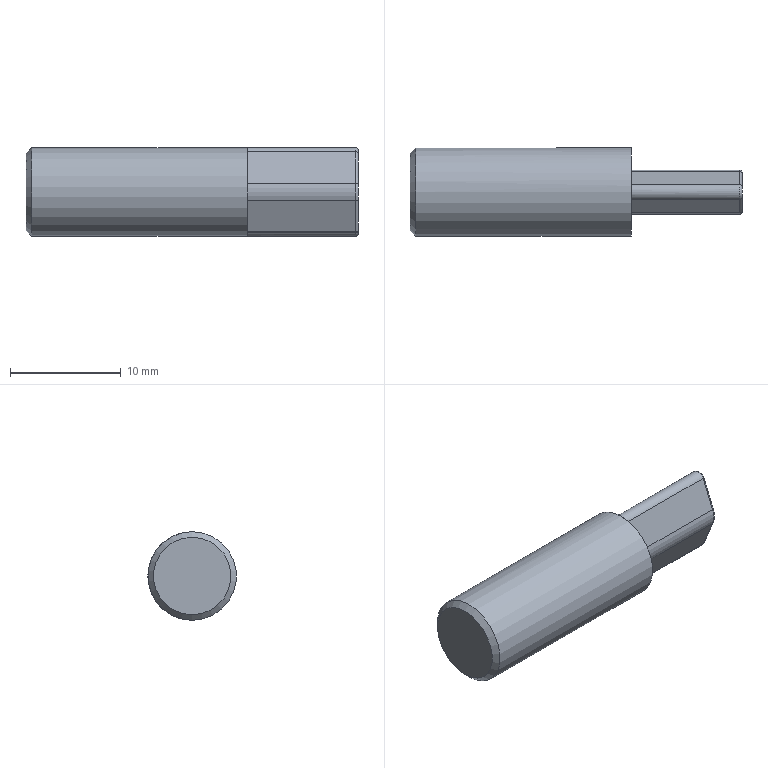Part | NX | features DATUM_CSYS 3, BLEND 2, EXTRUDE 2, SKETCH 2, CHAMFER 1 | 1 solid | 26 faces | box 30 x 8 x 8 mm | volume 1212 mm3 | cylinder 11 | plane 8 | torus 4 | sphere 2 | cone 1 | commonest cylinder face diameters 0.4 x6 1.5 x2 4 x2 8 x1
STEP:
#1=CARTESIAN_POINT('',(20.,0.,4.));
#2=VERTEX_POINT('',#1);
#3=CARTESIAN_POINT('',(20.,-0.6495,3.625));
#4=VERTEX_POINT('',#3);
#5=CARTESIAN_POINT('',(20.,0.,3.25));
#6=DIRECTION('',(1.,0.,0.));
#7=DIRECTION('',(0.,1.,0.));
#8=AXIS2_PLACEMENT_3D('',#5,#6,#7);
#9=CIRCLE('',#8,0.75);
#10=EDGE_CURVE('',#2,#4,#9,.T.);
#11=ORIENTED_EDGE('',*,*,#10,.F.);
#12=CARTESIAN_POINT('',(20.,0.,-4.));
#13=VERTEX_POINT('',#12);
#14=CARTESIAN_POINT('',(20.,0.,0.));
#15=DIRECTION('',(1.,0.,0.));
#16=DIRECTION('',(0.,1.,0.));
#17=AXIS2_PLACEMENT_3D('',#14,#15,#16);
#18=CIRCLE('',#17,4.);
#19=EDGE_CURVE('',#2,#13,#18,.T.);
#20=ORIENTED_EDGE('',*,*,#19,.T.);
#21=CARTESIAN_POINT('',(20.,-0.6414,-3.639));
#22=VERTEX_POINT('',#21);
#23=CARTESIAN_POINT('',(20.,0.,-3.25));
#24=DIRECTION('',(1.,0.,0.));
#25=DIRECTION('',(0.,1.,0.));
#26=AXIS2_PLACEMENT_3D('',#23,#24,#25);
#27=CIRCLE('',#26,0.75);
#28=EDGE_CURVE('',#22,#13,#27,.T.);
#29=ORIENTED_EDGE('',*,*,#28,.F.);
#30=CARTESIAN_POINT('',(20.,-0.6548,-3.612));
#31=VERTEX_POINT('',#30);
#32=CARTESIAN_POINT('',(20.,-0.4703,-3.535));
#33=DIRECTION('',(1.,0.,0.));
#34=DIRECTION('',(0.,0.,-1.));
#35=AXIS2_PLACEMENT_3D('',#32,#33,#34);
#36=CIRCLE('',#35,0.2);
#37=EDGE_CURVE('',#22,#31,#36,.F.);
#38=ORIENTED_EDGE('',*,*,#37,.T.);
#39=CARTESIAN_POINT('',(20.,-1.845,-0.7729));
#40=VERTEX_POINT('',#39);
#41=CARTESIAN_POINT('',(20.,-1.845,-0.7729));
#42=DIRECTION('',(0.,0.3865,-0.9223));
#43=VECTOR('',#42,1000.);
#44=LINE('',#41,#43);
#45=EDGE_CURVE('',#40,#31,#44,.T.);
#46=ORIENTED_EDGE('',*,*,#45,.F.);
#47=CARTESIAN_POINT('',(20.,-1.845,0.7729));
#48=VERTEX_POINT('',#47);
#49=CARTESIAN_POINT('',(20.,0.,0.));
#50=DIRECTION('',(1.,0.,0.));
#51=DIRECTION('',(0.,1.,0.));
#52=AXIS2_PLACEMENT_3D('',#49,#50,#51);
#53=CIRCLE('',#52,2.);
#54=EDGE_CURVE('',#48,#40,#53,.T.);
#55=ORIENTED_EDGE('',*,*,#54,.F.);
#56=CARTESIAN_POINT('',(20.,-0.6495,3.625));
#57=DIRECTION('',(0.,-0.3865,-0.9223));
#58=VECTOR('',#57,1000.);
#59=LINE('',#56,#58);
#60=EDGE_CURVE('',#4,#48,#59,.T.);
#61=ORIENTED_EDGE('',*,*,#60,.F.);
#62=EDGE_LOOP('',(#11,#20,#29,#38,#46,#55,#61));
#63=FACE_BOUND('',#62,.T.);
#64=CARTESIAN_POINT('',(20.,0.,0.));
#65=DIRECTION('',(1.,0.,0.));
#66=DIRECTION('',(0.,0.,-1.));
#67=AXIS2_PLACEMENT_3D('',#64,#65,#66);
#68=PLANE('',#67);
#69=ADVANCED_FACE('',(#63),#68,.T.);
#70=CARTESIAN_POINT('',(0.5,0.,-4.));
#71=VERTEX_POINT('',#70);
#72=CARTESIAN_POINT('',(0.5,0.,0.));
#73=DIRECTION('',(1.,0.,0.));
#74=DIRECTION('',(0.,0.,-1.));
#75=AXIS2_PLACEMENT_3D('',#72,#73,#74);
#76=CIRCLE('',#75,4.);
#77=EDGE_CURVE('',#71,#71,#76,.T.);
#78=ORIENTED_EDGE('',*,*,#77,.T.);
#79=EDGE_LOOP('',(#78));
#80=FACE_BOUND('',#79,.T.);
#81=ORIENTED_EDGE('',*,*,#19,.F.);
#82=CARTESIAN_POINT('',(20.,0.,0.));
#83=DIRECTION('',(1.,0.,0.));
#84=DIRECTION('',(0.,1.,0.));
#85=AXIS2_PLACEMENT_3D('',#82,#83,#84);
#86=CIRCLE('',#85,4.);
#87=EDGE_CURVE('',#13,#2,#86,.T.);
#88=ORIENTED_EDGE('',*,*,#87,.F.);
#89=EDGE_LOOP('',(#81,#88));
#90=FACE_BOUND('',#89,.T.);
#91=CARTESIAN_POINT('',(20.,0.,0.));
#92=DIRECTION('',(-1.,0.,0.));
#93=DIRECTION('',(0.,0.,1.));
#94=AXIS2_PLACEMENT_3D('',#91,#92,#93);
#95=CYLINDRICAL_SURFACE('',#94,4.);
#96=ADVANCED_FACE('',(#80,#90),#95,.T.);
#97=CARTESIAN_POINT('',(20.,0.6495,3.625));
#98=VERTEX_POINT('',#97);
#99=CARTESIAN_POINT('',(20.,0.,3.25));
#100=DIRECTION('',(1.,0.,0.));
#101=DIRECTION('',(0.,1.,0.));
#102=AXIS2_PLACEMENT_3D('',#99,#100,#101);
#103=CIRCLE('',#102,0.75);
#104=EDGE_CURVE('',#98,#2,#103,.T.);
#105=ORIENTED_EDGE('',*,*,#104,.F.);
#106=CARTESIAN_POINT('',(20.,1.845,0.7729));
#107=VERTEX_POINT('',#106);
#108=CARTESIAN_POINT('',(20.,1.845,0.7729));
#109=DIRECTION('',(0.,-0.3865,0.9223));
#110=VECTOR('',#109,1000.);
#111=LINE('',#108,#110);
#112=EDGE_CURVE('',#107,#98,#111,.T.);
#113=ORIENTED_EDGE('',*,*,#112,.F.);
#114=CARTESIAN_POINT('',(20.,1.845,-0.7729));
#115=VERTEX_POINT('',#114);
#116=CARTESIAN_POINT('',(20.,0.,0.));
#117=DIRECTION('',(1.,0.,0.));
#118=DIRECTION('',(0.,1.,0.));
#119=AXIS2_PLACEMENT_3D('',#116,#117,#118);
#120=CIRCLE('',#119,2.);
#121=EDGE_CURVE('',#115,#107,#120,.T.);
#122=ORIENTED_EDGE('',*,*,#121,.F.);
#123=CARTESIAN_POINT('',(20.,0.6548,-3.612));
#124=VERTEX_POINT('',#123);
#125=CARTESIAN_POINT('',(20.,0.6495,-3.625));
#126=DIRECTION('',(0.,0.3865,0.9223));
#127=VECTOR('',#126,1000.);
#128=LINE('',#125,#127);
#129=EDGE_CURVE('',#124,#115,#128,.T.);
#130=ORIENTED_EDGE('',*,*,#129,.F.);
#131=CARTESIAN_POINT('',(20.,0.6414,-3.639));
#132=VERTEX_POINT('',#131);
#133=CARTESIAN_POINT('',(20.,0.4703,-3.535));
#134=DIRECTION('',(1.,0.,0.));
#135=DIRECTION('',(0.,0.,-1.));
#136=AXIS2_PLACEMENT_3D('',#133,#134,#135);
#137=CIRCLE('',#136,0.2);
#138=EDGE_CURVE('',#124,#132,#137,.F.);
#139=ORIENTED_EDGE('',*,*,#138,.T.);
#140=CARTESIAN_POINT('',(20.,0.,-3.25));
#141=DIRECTION('',(1.,0.,0.));
#142=DIRECTION('',(0.,1.,0.));
#143=AXIS2_PLACEMENT_3D('',#140,#141,#142);
#144=CIRCLE('',#143,0.75);
#145=EDGE_CURVE('',#13,#132,#144,.T.);
#146=ORIENTED_EDGE('',*,*,#145,.F.);
#147=ORIENTED_EDGE('',*,*,#87,.T.);
#148=EDGE_LOOP('',(#105,#113,#122,#130,#139,#146,#147));
#149=FACE_BOUND('',#148,.T.);
#150=CARTESIAN_POINT('',(20.,0.,0.));
#151=DIRECTION('',(1.,0.,0.));
#152=DIRECTION('',(0.,0.,-1.));
#153=AXIS2_PLACEMENT_3D('',#150,#151,#152);
#154=PLANE('',#153);
#155=ADVANCED_FACE('',(#149),#154,.T.);
#156=CARTESIAN_POINT('',(0.,0.,-3.5));
#157=VERTEX_POINT('',#156);
#158=CARTESIAN_POINT('',(0.,0.,0.));
#159=DIRECTION('',(1.,0.,0.));
#160=DIRECTION('',(0.,0.,-1.));
#161=AXIS2_PLACEMENT_3D('',#158,#159,#160);
#162=CIRCLE('',#161,3.5);
#163=EDGE_CURVE('',#157,#157,#162,.F.);
#164=ORIENTED_EDGE('',*,*,#163,.T.);
#165=EDGE_LOOP('',(#164));
#166=FACE_BOUND('',#165,.T.);
#167=CARTESIAN_POINT('',(0.,0.,0.));
#168=DIRECTION('',(1.,0.,0.));
#169=DIRECTION('',(0.,0.,-1.));
#170=AXIS2_PLACEMENT_3D('',#167,#168,#169);
#171=PLANE('',#170);
#172=ADVANCED_FACE('',(#166),#171,.F.);
#173=ORIENTED_EDGE('',*,*,#163,.F.);
#174=EDGE_LOOP('',(#173));
#175=FACE_BOUND('',#174,.T.);
#176=ORIENTED_EDGE('',*,*,#77,.F.);
#177=EDGE_LOOP('',(#176));
#178=FACE_BOUND('',#177,.T.);
#179=CARTESIAN_POINT('',(0.5,0.,0.));
#180=DIRECTION('',(1.,0.,0.));
#181=DIRECTION('',(0.,0.,-1.));
#182=AXIS2_PLACEMENT_3D('',#179,#180,#181);
#183=CONICAL_SURFACE('',#182,4.,0.7854);
#184=ADVANCED_FACE('',(#175,#178),#183,.T.);
#185=CARTESIAN_POINT('',(29.8,-1.845,-0.7729));
#186=VERTEX_POINT('',#185);
#187=CARTESIAN_POINT('',(30.,-1.845,-0.7729));
#188=DIRECTION('',(-1.,0.,0.));
#189=VECTOR('',#188,1000.);
#190=LINE('',#187,#189);
#191=EDGE_CURVE('',#186,#40,#190,.T.);
#192=ORIENTED_EDGE('',*,*,#191,.F.);
#193=CARTESIAN_POINT('',(29.8,-1.845,0.7729));
#194=VERTEX_POINT('',#193);
#195=CARTESIAN_POINT('',(29.8,0.,0.));
#196=DIRECTION('',(1.,0.,0.));
#197=DIRECTION('',(0.,0.,-1.));
#198=AXIS2_PLACEMENT_3D('',#195,#196,#197);
#199=CIRCLE('',#198,2.);
#200=EDGE_CURVE('',#186,#194,#199,.F.);
#201=ORIENTED_EDGE('',*,*,#200,.T.);
#202=CARTESIAN_POINT('',(30.,-1.845,0.7729));
#203=DIRECTION('',(-1.,0.,0.));
#204=VECTOR('',#203,1000.);
#205=LINE('',#202,#204);
#206=EDGE_CURVE('',#194,#48,#205,.T.);
#207=ORIENTED_EDGE('',*,*,#206,.T.);
#208=ORIENTED_EDGE('',*,*,#54,.T.);
#209=EDGE_LOOP('',(#192,#201,#207,#208));
#210=FACE_BOUND('',#209,.T.);
#211=CARTESIAN_POINT('',(30.,0.,0.));
#212=DIRECTION('',(-1.,0.,0.));
#213=DIRECTION('',(0.,0.,1.));
#214=AXIS2_PLACEMENT_3D('',#211,#212,#213);
#215=CYLINDRICAL_SURFACE('',#214,2.);
#216=ADVANCED_FACE('',(#210),#215,.T.);
#217=ORIENTED_EDGE('',*,*,#45,.T.);
#218=CARTESIAN_POINT('',(29.8,-0.6548,-3.612));
#219=VERTEX_POINT('',#218);
#220=CARTESIAN_POINT('',(30.,-0.6548,-3.612));
#221=DIRECTION('',(-1.,0.,0.));
#222=VECTOR('',#221,1000.);
#223=LINE('',#220,#222);
#224=EDGE_CURVE('',#31,#219,#223,.F.);
#225=ORIENTED_EDGE('',*,*,#224,.T.);
#226=CARTESIAN_POINT('',(29.8,-1.845,-0.7729));
#227=DIRECTION('',(0.,0.3865,-0.9223));
#228=VECTOR('',#227,1000.);
#229=LINE('',#226,#228);
#230=EDGE_CURVE('',#219,#186,#229,.F.);
#231=ORIENTED_EDGE('',*,*,#230,.T.);
#232=ORIENTED_EDGE('',*,*,#191,.T.);
#233=EDGE_LOOP('',(#217,#225,#231,#232));
#234=FACE_BOUND('',#233,.T.);
#235=CARTESIAN_POINT('',(30.,-1.845,-0.7729));
#236=DIRECTION('',(0.,0.9223,0.3865));
#237=DIRECTION('',(0.,-0.3865,0.9223));
#238=AXIS2_PLACEMENT_3D('',#235,#236,#237);
#239=PLANE('',#238);
#240=ADVANCED_FACE('',(#234),#239,.F.);
#241=CARTESIAN_POINT('',(29.8,0.6414,-3.639));
#242=VERTEX_POINT('',#241);
#243=CARTESIAN_POINT('',(29.8,-0.6414,-3.639));
#244=VERTEX_POINT('',#243);
#245=CARTESIAN_POINT('',(29.8,0.,-3.25));
#246=DIRECTION('',(1.,0.,0.));
#247=DIRECTION('',(0.,0.,-1.));
#248=AXIS2_PLACEMENT_3D('',#245,#246,#247);
#249=CIRCLE('',#248,0.75);
#250=EDGE_CURVE('',#242,#244,#249,.F.);
#251=ORIENTED_EDGE('',*,*,#250,.T.);
#252=CARTESIAN_POINT('',(30.,-0.6414,-3.639));
#253=DIRECTION('',(-1.,0.,0.));
#254=VECTOR('',#253,1000.);
#255=LINE('',#252,#254);
#256=EDGE_CURVE('',#244,#22,#255,.T.);
#257=ORIENTED_EDGE('',*,*,#256,.T.);
#258=ORIENTED_EDGE('',*,*,#28,.T.);
#259=ORIENTED_EDGE('',*,*,#145,.T.);
#260=CARTESIAN_POINT('',(30.,0.6414,-3.639));
#261=DIRECTION('',(-1.,0.,0.));
#262=VECTOR('',#261,1000.);
#263=LINE('',#260,#262);
#264=EDGE_CURVE('',#132,#242,#263,.F.);
#265=ORIENTED_EDGE('',*,*,#264,.T.);
#266=EDGE_LOOP('',(#251,#257,#258,#259,#265));
#267=FACE_BOUND('',#266,.T.);
#268=CARTESIAN_POINT('',(30.,0.,-3.25));
#269=DIRECTION('',(-1.,0.,0.));
#270=DIRECTION('',(0.,0.,1.));
#271=AXIS2_PLACEMENT_3D('',#268,#269,#270);
#272=CYLINDRICAL_SURFACE('',#271,0.75);
#273=ADVANCED_FACE('',(#267),#272,.T.);
#274=CARTESIAN_POINT('',(29.8,1.845,-0.7729));
#275=VERTEX_POINT('',#274);
#276=CARTESIAN_POINT('',(29.8,0.6548,-3.612));
#277=VERTEX_POINT('',#276);
#278=CARTESIAN_POINT('',(29.8,0.6495,-3.625));
#279=DIRECTION('',(0.,0.3865,0.9223));
#280=VECTOR('',#279,1000.);
#281=LINE('',#278,#280);
#282=EDGE_CURVE('',#275,#277,#281,.F.);
#283=ORIENTED_EDGE('',*,*,#282,.T.);
#284=CARTESIAN_POINT('',(30.,0.6548,-3.612));
#285=DIRECTION('',(-1.,0.,0.));
#286=VECTOR('',#285,1000.);
#287=LINE('',#284,#286);
#288=EDGE_CURVE('',#277,#124,#287,.T.);
#289=ORIENTED_EDGE('',*,*,#288,.T.);
#290=ORIENTED_EDGE('',*,*,#129,.T.);
#291=CARTESIAN_POINT('',(30.,1.845,-0.7729));
#292=DIRECTION('',(-1.,0.,0.));
#293=VECTOR('',#292,1000.);
#294=LINE('',#291,#293);
#295=EDGE_CURVE('',#275,#115,#294,.T.);
#296=ORIENTED_EDGE('',*,*,#295,.F.);
#297=EDGE_LOOP('',(#283,#289,#290,#296));
#298=FACE_BOUND('',#297,.T.);
#299=CARTESIAN_POINT('',(30.,0.6495,-3.625));
#300=DIRECTION('',(0.,-0.9223,0.3865));
#301=DIRECTION('',(0.,-0.3865,-0.9223));
#302=AXIS2_PLACEMENT_3D('',#299,#300,#301);
#303=PLANE('',#302);
#304=ADVANCED_FACE('',(#298),#303,.F.);
#305=CARTESIAN_POINT('',(29.8,1.845,0.7729));
#306=VERTEX_POINT('',#305);
#307=CARTESIAN_POINT('',(30.,1.845,0.7729));
#308=DIRECTION('',(-1.,0.,0.));
#309=VECTOR('',#308,1000.);
#310=LINE('',#307,#309);
#311=EDGE_CURVE('',#306,#107,#310,.T.);
#312=ORIENTED_EDGE('',*,*,#311,.F.);
#313=CARTESIAN_POINT('',(29.8,0.,0.));
#314=DIRECTION('',(1.,0.,0.));
#315=DIRECTION('',(0.,0.,-1.));
#316=AXIS2_PLACEMENT_3D('',#313,#314,#315);
#317=CIRCLE('',#316,2.);
#318=EDGE_CURVE('',#306,#275,#317,.F.);
#319=ORIENTED_EDGE('',*,*,#318,.T.);
#320=ORIENTED_EDGE('',*,*,#295,.T.);
#321=ORIENTED_EDGE('',*,*,#121,.T.);
#322=EDGE_LOOP('',(#312,#319,#320,#321));
#323=FACE_BOUND('',#322,.T.);
#324=CARTESIAN_POINT('',(30.,0.,0.));
#325=DIRECTION('',(-1.,0.,0.));
#326=DIRECTION('',(0.,0.,1.));
#327=AXIS2_PLACEMENT_3D('',#324,#325,#326);
#328=CYLINDRICAL_SURFACE('',#327,2.);
#329=ADVANCED_FACE('',(#323),#328,.T.);
#330=CARTESIAN_POINT('',(29.8,0.6495,3.625));
#331=VERTEX_POINT('',#330);
#332=CARTESIAN_POINT('',(30.,0.6495,3.625));
#333=DIRECTION('',(-1.,0.,0.));
#334=VECTOR('',#333,1000.);
#335=LINE('',#332,#334);
#336=EDGE_CURVE('',#331,#98,#335,.T.);
#337=ORIENTED_EDGE('',*,*,#336,.F.);
#338=CARTESIAN_POINT('',(29.8,1.845,0.7729));
#339=DIRECTION('',(0.,-0.3865,0.9223));
#340=VECTOR('',#339,1000.);
#341=LINE('',#338,#340);
#342=EDGE_CURVE('',#331,#306,#341,.F.);
#343=ORIENTED_EDGE('',*,*,#342,.T.);
#344=ORIENTED_EDGE('',*,*,#311,.T.);
#345=ORIENTED_EDGE('',*,*,#112,.T.);
#346=EDGE_LOOP('',(#337,#343,#344,#345));
#347=FACE_BOUND('',#346,.T.);
#348=CARTESIAN_POINT('',(30.,1.845,0.7729));
#349=DIRECTION('',(0.,-0.9223,-0.3865));
#350=DIRECTION('',(0.,0.3865,-0.9223));
#351=AXIS2_PLACEMENT_3D('',#348,#349,#350);
#352=PLANE('',#351);
#353=ADVANCED_FACE('',(#347),#352,.F.);
#354=CARTESIAN_POINT('',(29.8,-0.6495,3.625));
#355=VERTEX_POINT('',#354);
#356=CARTESIAN_POINT('',(30.,-0.6495,3.625));
#357=DIRECTION('',(-1.,0.,0.));
#358=VECTOR('',#357,1000.);
#359=LINE('',#356,#358);
#360=EDGE_CURVE('',#355,#4,#359,.T.);
#361=ORIENTED_EDGE('',*,*,#360,.F.);
#362=CARTESIAN_POINT('',(29.8,0.,3.25));
#363=DIRECTION('',(1.,0.,0.));
#364=DIRECTION('',(0.,0.,-1.));
#365=AXIS2_PLACEMENT_3D('',#362,#363,#364);
#366=CIRCLE('',#365,0.75);
#367=EDGE_CURVE('',#355,#331,#366,.F.);
#368=ORIENTED_EDGE('',*,*,#367,.T.);
#369=ORIENTED_EDGE('',*,*,#336,.T.);
#370=ORIENTED_EDGE('',*,*,#104,.T.);
#371=ORIENTED_EDGE('',*,*,#10,.T.);
#372=EDGE_LOOP('',(#361,#368,#369,#370,#371));
#373=FACE_BOUND('',#372,.T.);
#374=CARTESIAN_POINT('',(30.,0.,3.25));
#375=DIRECTION('',(-1.,0.,0.));
#376=DIRECTION('',(0.,0.,1.));
#377=AXIS2_PLACEMENT_3D('',#374,#375,#376);
#378=CYLINDRICAL_SURFACE('',#377,0.75);
#379=ADVANCED_FACE('',(#373),#378,.T.);
#380=ORIENTED_EDGE('',*,*,#206,.F.);
#381=CARTESIAN_POINT('',(29.8,-0.6495,3.625));
#382=DIRECTION('',(0.,-0.3865,-0.9223));
#383=VECTOR('',#382,1000.);
#384=LINE('',#381,#383);
#385=EDGE_CURVE('',#194,#355,#384,.F.);
#386=ORIENTED_EDGE('',*,*,#385,.T.);
#387=ORIENTED_EDGE('',*,*,#360,.T.);
#388=ORIENTED_EDGE('',*,*,#60,.T.);
#389=EDGE_LOOP('',(#380,#386,#387,#388));
#390=FACE_BOUND('',#389,.T.);
#391=CARTESIAN_POINT('',(30.,-0.6495,3.625));
#392=DIRECTION('',(0.,0.9223,-0.3865));
#393=DIRECTION('',(0.,0.3865,0.9223));
#394=AXIS2_PLACEMENT_3D('',#391,#392,#393);
#395=PLANE('',#394);
#396=ADVANCED_FACE('',(#390),#395,.F.);
#397=CARTESIAN_POINT('',(30.,-1.66,-0.6956));
#398=VERTEX_POINT('',#397);
#399=CARTESIAN_POINT('',(30.,-0.4703,-3.535));
#400=VERTEX_POINT('',#399);
#401=CARTESIAN_POINT('',(30.,-0.4651,-3.548));
#402=DIRECTION('',(0.,0.3865,-0.9223));
#403=VECTOR('',#402,1000.);
#404=LINE('',#401,#403);
#405=EDGE_CURVE('',#398,#400,#404,.T.);
#406=ORIENTED_EDGE('',*,*,#405,.T.);
#407=CARTESIAN_POINT('',(30.,0.4703,-3.535));
#408=VERTEX_POINT('',#407);
#409=CARTESIAN_POINT('',(30.,0.,-3.25));
#410=DIRECTION('',(1.,0.,0.));
#411=DIRECTION('',(0.,0.,-1.));
#412=AXIS2_PLACEMENT_3D('',#409,#410,#411);
#413=CIRCLE('',#412,0.55);
#414=EDGE_CURVE('',#400,#408,#413,.T.);
#415=ORIENTED_EDGE('',*,*,#414,.T.);
#416=CARTESIAN_POINT('',(30.,1.66,-0.6956));
#417=VERTEX_POINT('',#416);
#418=CARTESIAN_POINT('',(30.,1.66,-0.6956));
#419=DIRECTION('',(0.,0.3865,0.9223));
#420=VECTOR('',#419,1000.);
#421=LINE('',#418,#420);
#422=EDGE_CURVE('',#408,#417,#421,.T.);
#423=ORIENTED_EDGE('',*,*,#422,.T.);
#424=CARTESIAN_POINT('',(30.,1.66,0.6956));
#425=VERTEX_POINT('',#424);
#426=CARTESIAN_POINT('',(30.,0.,0.));
#427=DIRECTION('',(1.,0.,0.));
#428=DIRECTION('',(0.,0.,-1.));
#429=AXIS2_PLACEMENT_3D('',#426,#427,#428);
#430=CIRCLE('',#429,1.8);
#431=EDGE_CURVE('',#417,#425,#430,.T.);
#432=ORIENTED_EDGE('',*,*,#431,.T.);
#433=CARTESIAN_POINT('',(30.,0.4703,3.535));
#434=VERTEX_POINT('',#433);
#435=CARTESIAN_POINT('',(30.,0.4651,3.548));
#436=DIRECTION('',(0.,-0.3865,0.9223));
#437=VECTOR('',#436,1000.);
#438=LINE('',#435,#437);
#439=EDGE_CURVE('',#425,#434,#438,.T.);
#440=ORIENTED_EDGE('',*,*,#439,.T.);
#441=CARTESIAN_POINT('',(30.,-0.4703,3.535));
#442=VERTEX_POINT('',#441);
#443=CARTESIAN_POINT('',(30.,0.,3.25));
#444=DIRECTION('',(1.,0.,0.));
#445=DIRECTION('',(0.,0.,-1.));
#446=AXIS2_PLACEMENT_3D('',#443,#444,#445);
#447=CIRCLE('',#446,0.55);
#448=EDGE_CURVE('',#434,#442,#447,.T.);
#449=ORIENTED_EDGE('',*,*,#448,.T.);
#450=CARTESIAN_POINT('',(30.,-1.66,0.6956));
#451=VERTEX_POINT('',#450);
#452=CARTESIAN_POINT('',(30.,-1.66,0.6956));
#453=DIRECTION('',(0.,-0.3865,-0.9223));
#454=VECTOR('',#453,1000.);
#455=LINE('',#452,#454);
#456=EDGE_CURVE('',#442,#451,#455,.T.);
#457=ORIENTED_EDGE('',*,*,#456,.T.);
#458=CARTESIAN_POINT('',(30.,0.,0.));
#459=DIRECTION('',(1.,0.,0.));
#460=DIRECTION('',(0.,0.,-1.));
#461=AXIS2_PLACEMENT_3D('',#458,#459,#460);
#462=CIRCLE('',#461,1.8);
#463=EDGE_CURVE('',#451,#398,#462,.T.);
#464=ORIENTED_EDGE('',*,*,#463,.T.);
#465=EDGE_LOOP('',(#406,#415,#423,#432,#440,#449,#457,#464));
#466=FACE_BOUND('',#465,.T.);
#467=CARTESIAN_POINT('',(30.,0.,0.));
#468=DIRECTION('',(1.,0.,0.));
#469=DIRECTION('',(0.,0.,-1.));
#470=AXIS2_PLACEMENT_3D('',#467,#468,#469);
#471=PLANE('',#470);
#472=ADVANCED_FACE('',(#466),#471,.T.);
#473=ORIENTED_EDGE('',*,*,#230,.F.);
#474=CARTESIAN_POINT('',(29.8,-0.4703,-3.535));
#475=DIRECTION('',(0.,-0.3865,0.9223));
#476=DIRECTION('',(0.,-0.9223,-0.3865));
#477=AXIS2_PLACEMENT_3D('',#474,#475,#476);
#478=CIRCLE('',#477,0.2);
#479=EDGE_CURVE('',#219,#400,#478,.T.);
#480=ORIENTED_EDGE('',*,*,#479,.T.);
#481=ORIENTED_EDGE('',*,*,#405,.F.);
#482=CARTESIAN_POINT('',(29.8,-1.66,-0.6956));
#483=DIRECTION('',(0.,-0.3865,0.9223));
#484=DIRECTION('',(0.,-0.9223,-0.3865));
#485=AXIS2_PLACEMENT_3D('',#482,#483,#484);
#486=CIRCLE('',#485,0.2);
#487=EDGE_CURVE('',#186,#398,#486,.T.);
#488=ORIENTED_EDGE('',*,*,#487,.F.);
#489=EDGE_LOOP('',(#473,#480,#481,#488));
#490=FACE_BOUND('',#489,.T.);
#491=CARTESIAN_POINT('',(29.8,-1.66,-0.6956));
#492=DIRECTION('',(0.,-0.3865,0.9223));
#493=DIRECTION('',(0.,-0.9223,-0.3865));
#494=AXIS2_PLACEMENT_3D('',#491,#492,#493);
#495=CYLINDRICAL_SURFACE('',#494,0.2);
#496=ADVANCED_FACE('',(#490),#495,.T.);
#497=ORIENTED_EDGE('',*,*,#487,.T.);
#498=ORIENTED_EDGE('',*,*,#463,.F.);
#499=CARTESIAN_POINT('',(29.8,-1.66,0.6956));
#500=DIRECTION('',(0.,0.3865,0.9223));
#501=DIRECTION('',(0.,-0.9223,0.3865));
#502=AXIS2_PLACEMENT_3D('',#499,#500,#501);
#503=CIRCLE('',#502,0.2);
#504=EDGE_CURVE('',#194,#451,#503,.T.);
#505=ORIENTED_EDGE('',*,*,#504,.F.);
#506=ORIENTED_EDGE('',*,*,#200,.F.);
#507=EDGE_LOOP('',(#497,#498,#505,#506));
#508=FACE_BOUND('',#507,.T.);
#509=CARTESIAN_POINT('',(29.8,0.,0.));
#510=DIRECTION('',(1.,0.,0.));
#511=DIRECTION('',(0.,0.,-1.));
#512=AXIS2_PLACEMENT_3D('',#509,#510,#511);
#513=TOROIDAL_SURFACE('',#512,1.8,0.2);
#514=ADVANCED_FACE('',(#508),#513,.T.);
#515=ORIENTED_EDGE('',*,*,#422,.F.);
#516=CARTESIAN_POINT('',(29.8,0.4703,-3.535));
#517=DIRECTION('',(0.,-0.3865,-0.9223));
#518=DIRECTION('',(0.,0.9223,-0.3865));
#519=AXIS2_PLACEMENT_3D('',#516,#517,#518);
#520=CIRCLE('',#519,0.2);
#521=EDGE_CURVE('',#408,#277,#520,.F.);
#522=ORIENTED_EDGE('',*,*,#521,.T.);
#523=ORIENTED_EDGE('',*,*,#282,.F.);
#524=CARTESIAN_POINT('',(29.8,1.66,-0.6956));
#525=DIRECTION('',(0.,0.3865,0.9223));
#526=DIRECTION('',(0.,-0.9223,0.3865));
#527=AXIS2_PLACEMENT_3D('',#524,#525,#526);
#528=CIRCLE('',#527,0.2);
#529=EDGE_CURVE('',#417,#275,#528,.T.);
#530=ORIENTED_EDGE('',*,*,#529,.F.);
#531=EDGE_LOOP('',(#515,#522,#523,#530));
#532=FACE_BOUND('',#531,.T.);
#533=CARTESIAN_POINT('',(29.8,1.66,-0.6956));
#534=DIRECTION('',(0.,-0.3865,-0.9223));
#535=DIRECTION('',(0.,0.9223,-0.3865));
#536=AXIS2_PLACEMENT_3D('',#533,#534,#535);
#537=CYLINDRICAL_SURFACE('',#536,0.2);
#538=ADVANCED_FACE('',(#532),#537,.T.);
#539=ORIENTED_EDGE('',*,*,#504,.T.);
#540=ORIENTED_EDGE('',*,*,#456,.F.);
#541=CARTESIAN_POINT('',(29.8,-0.6495,3.625));
#542=CARTESIAN_POINT('',(29.906,-0.6495,3.625));
#543=CARTESIAN_POINT('',(30.,-0.5633,3.582));
#544=CARTESIAN_POINT('',(30.,-0.4703,3.535));
#545=B_SPLINE_CURVE_WITH_KNOTS('',3,(#541,#542,#543,#544),.UNSPECIFIED.,.F.,.F.,(4,4),(0.,0.0003128),.UNSPECIFIED.);
#546=EDGE_CURVE('',#355,#442,#545,.T.);
#547=ORIENTED_EDGE('',*,*,#546,.F.);
#548=ORIENTED_EDGE('',*,*,#385,.F.);
#549=EDGE_LOOP('',(#539,#540,#547,#548));
#550=FACE_BOUND('',#549,.T.);
#551=CARTESIAN_POINT('',(29.8,-1.66,0.6956));
#552=DIRECTION('',(0.,0.3865,0.9223));
#553=DIRECTION('',(0.,-0.9223,0.3865));
#554=AXIS2_PLACEMENT_3D('',#551,#552,#553);
#555=CYLINDRICAL_SURFACE('',#554,0.2);
#556=ADVANCED_FACE('',(#550),#555,.T.);
#557=ORIENTED_EDGE('',*,*,#529,.T.);
#558=ORIENTED_EDGE('',*,*,#318,.F.);
#559=CARTESIAN_POINT('',(29.8,1.66,0.6956));
#560=DIRECTION('',(0.,-0.3865,0.9223));
#561=DIRECTION('',(0.,-0.9223,-0.3865));
#562=AXIS2_PLACEMENT_3D('',#559,#560,#561);
#563=CIRCLE('',#562,0.2);
#564=EDGE_CURVE('',#425,#306,#563,.T.);
#565=ORIENTED_EDGE('',*,*,#564,.F.);
#566=ORIENTED_EDGE('',*,*,#431,.F.);
#567=EDGE_LOOP('',(#557,#558,#565,#566));
#568=FACE_BOUND('',#567,.T.);
#569=CARTESIAN_POINT('',(29.8,0.,0.));
#570=DIRECTION('',(1.,0.,0.));
#571=DIRECTION('',(0.,0.,-1.));
#572=AXIS2_PLACEMENT_3D('',#569,#570,#571);
#573=TOROIDAL_SURFACE('',#572,1.8,0.2);
#574=ADVANCED_FACE('',(#568),#573,.T.);
#575=ORIENTED_EDGE('',*,*,#546,.T.);
#576=ORIENTED_EDGE('',*,*,#448,.F.);
#577=CARTESIAN_POINT('',(29.8,0.6495,3.625));
#578=CARTESIAN_POINT('',(29.906,0.6495,3.625));
#579=CARTESIAN_POINT('',(30.,0.5633,3.582));
#580=CARTESIAN_POINT('',(30.,0.4703,3.535));
#581=B_SPLINE_CURVE_WITH_KNOTS('',3,(#577,#578,#579,#580),.UNSPECIFIED.,.F.,.F.,(4,4),(0.,0.0003128),.UNSPECIFIED.);
#582=EDGE_CURVE('',#331,#434,#581,.T.);
#583=ORIENTED_EDGE('',*,*,#582,.F.);
#584=ORIENTED_EDGE('',*,*,#367,.F.);
#585=EDGE_LOOP('',(#575,#576,#583,#584));
#586=FACE_BOUND('',#585,.T.);
#587=CARTESIAN_POINT('',(29.8,0.,3.25));
#588=DIRECTION('',(1.,0.,0.));
#589=DIRECTION('',(0.,0.,-1.));
#590=AXIS2_PLACEMENT_3D('',#587,#588,#589);
#591=TOROIDAL_SURFACE('',#590,0.55,0.2);
#592=ADVANCED_FACE('',(#586),#591,.T.);
#593=ORIENTED_EDGE('',*,*,#564,.T.);
#594=ORIENTED_EDGE('',*,*,#342,.F.);
#595=ORIENTED_EDGE('',*,*,#582,.T.);
#596=ORIENTED_EDGE('',*,*,#439,.F.);
#597=EDGE_LOOP('',(#593,#594,#595,#596));
#598=FACE_BOUND('',#597,.T.);
#599=CARTESIAN_POINT('',(29.8,1.66,0.6956));
#600=DIRECTION('',(0.,0.3865,-0.9223));
#601=DIRECTION('',(0.,0.9223,0.3865));
#602=AXIS2_PLACEMENT_3D('',#599,#600,#601);
#603=CYLINDRICAL_SURFACE('',#602,0.2);
#604=ADVANCED_FACE('',(#598),#603,.T.);
#605=ORIENTED_EDGE('',*,*,#138,.F.);
#606=ORIENTED_EDGE('',*,*,#288,.F.);
#607=CARTESIAN_POINT('',(29.8,0.4703,-3.535));
#608=DIRECTION('',(1.,0.,0.));
#609=DIRECTION('',(0.,0.,-1.));
#610=AXIS2_PLACEMENT_3D('',#607,#608,#609);
#611=CIRCLE('',#610,0.2);
#612=EDGE_CURVE('',#242,#277,#611,.T.);
#613=ORIENTED_EDGE('',*,*,#612,.F.);
#614=ORIENTED_EDGE('',*,*,#264,.F.);
#615=EDGE_LOOP('',(#605,#606,#613,#614));
#616=FACE_BOUND('',#615,.T.);
#617=CARTESIAN_POINT('',(30.,0.4703,-3.535));
#618=DIRECTION('',(-1.,0.,0.));
#619=DIRECTION('',(0.,0.,1.));
#620=AXIS2_PLACEMENT_3D('',#617,#618,#619);
#621=CYLINDRICAL_SURFACE('',#620,0.2);
#622=ADVANCED_FACE('',(#616),#621,.T.);
#623=ORIENTED_EDGE('',*,*,#612,.T.);
#624=ORIENTED_EDGE('',*,*,#521,.F.);
#625=CARTESIAN_POINT('',(29.8,0.4703,-3.535));
#626=DIRECTION('',(0.,-0.5183,-0.8552));
#627=DIRECTION('',(0.,0.8552,-0.5183));
#628=AXIS2_PLACEMENT_3D('',#625,#626,#627);
#629=CIRCLE('',#628,0.2);
#630=EDGE_CURVE('',#242,#408,#629,.T.);
#631=ORIENTED_EDGE('',*,*,#630,.F.);
#632=EDGE_LOOP('',(#623,#624,#631));
#633=FACE_BOUND('',#632,.T.);
#634=CARTESIAN_POINT('',(29.8,0.4703,-3.535));
#635=DIRECTION('',(0.,-0.8552,0.5183));
#636=DIRECTION('',(0.,-0.5183,-0.8552));
#637=AXIS2_PLACEMENT_3D('',#634,#635,#636);
#638=SPHERICAL_SURFACE('',#637,0.2);
#639=ADVANCED_FACE('',(#633),#638,.T.);
#640=ORIENTED_EDGE('',*,*,#630,.T.);
#641=ORIENTED_EDGE('',*,*,#414,.F.);
#642=CARTESIAN_POINT('',(29.8,-0.4703,-3.535));
#643=DIRECTION('',(0.,-0.5183,0.8552));
#644=DIRECTION('',(0.,-0.8552,-0.5183));
#645=AXIS2_PLACEMENT_3D('',#642,#643,#644);
#646=CIRCLE('',#645,0.2);
#647=EDGE_CURVE('',#244,#400,#646,.T.);
#648=ORIENTED_EDGE('',*,*,#647,.F.);
#649=ORIENTED_EDGE('',*,*,#250,.F.);
#650=EDGE_LOOP('',(#640,#641,#648,#649));
#651=FACE_BOUND('',#650,.T.);
#652=CARTESIAN_POINT('',(29.8,0.,-3.25));
#653=DIRECTION('',(1.,0.,0.));
#654=DIRECTION('',(0.,0.,-1.));
#655=AXIS2_PLACEMENT_3D('',#652,#653,#654);
#656=TOROIDAL_SURFACE('',#655,0.55,0.2);
#657=ADVANCED_FACE('',(#651),#656,.T.);
#658=ORIENTED_EDGE('',*,*,#647,.T.);
#659=ORIENTED_EDGE('',*,*,#479,.F.);
#660=CARTESIAN_POINT('',(29.8,-0.4703,-3.535));
#661=DIRECTION('',(-1.,0.,0.));
#662=DIRECTION('',(0.,0.,1.));
#663=AXIS2_PLACEMENT_3D('',#660,#661,#662);
#664=CIRCLE('',#663,0.2);
#665=EDGE_CURVE('',#244,#219,#664,.T.);
#666=ORIENTED_EDGE('',*,*,#665,.F.);
#667=EDGE_LOOP('',(#658,#659,#666));
#668=FACE_BOUND('',#667,.T.);
#669=CARTESIAN_POINT('',(29.8,-0.4703,-3.535));
#670=DIRECTION('',(0.,0.8552,0.5183));
#671=DIRECTION('',(0.,-0.5183,0.8552));
#672=AXIS2_PLACEMENT_3D('',#669,#670,#671);
#673=SPHERICAL_SURFACE('',#672,0.2);
#674=ADVANCED_FACE('',(#668),#673,.T.);
#675=ORIENTED_EDGE('',*,*,#665,.T.);
#676=ORIENTED_EDGE('',*,*,#224,.F.);
#677=ORIENTED_EDGE('',*,*,#37,.F.);
#678=ORIENTED_EDGE('',*,*,#256,.F.);
#679=EDGE_LOOP('',(#675,#676,#677,#678));
#680=FACE_BOUND('',#679,.T.);
#681=CARTESIAN_POINT('',(30.,-0.4703,-3.535));
#682=DIRECTION('',(-1.,0.,0.));
#683=DIRECTION('',(0.,0.,1.));
#684=AXIS2_PLACEMENT_3D('',#681,#682,#683);
#685=CYLINDRICAL_SURFACE('',#684,0.2);
#686=ADVANCED_FACE('',(#680),#685,.T.);
#687=CLOSED_SHELL('',(#69,#96,#155,#172,#184,#216,#240,#273,#304,#329,#353,#379,#396,#472,#496,#514,#538,#556,#574,#592,#604,#622,#639,#657,#674,#686));
#688=MANIFOLD_SOLID_BREP('',#687);
#689=(LENGTH_UNIT()NAMED_UNIT(*)SI_UNIT(.MILLI.,.METRE.));
#690=UNCERTAINTY_MEASURE_WITH_UNIT(LENGTH_MEASURE(0.0508),#689,'','');
#691=(NAMED_UNIT(*)PLANE_ANGLE_UNIT()SI_UNIT($,.RADIAN.));
#692=(NAMED_UNIT(*)SI_UNIT($,.STERADIAN.)SOLID_ANGLE_UNIT());
#693=(GEOMETRIC_REPRESENTATION_CONTEXT(3)GLOBAL_UNCERTAINTY_ASSIGNED_CONTEXT((#690))GLOBAL_UNIT_ASSIGNED_CONTEXT((#689,#691,#692))REPRESENTATION_CONTEXT('',''));
#694=ADVANCED_BREP_SHAPE_REPRESENTATION('',(#688),#693);